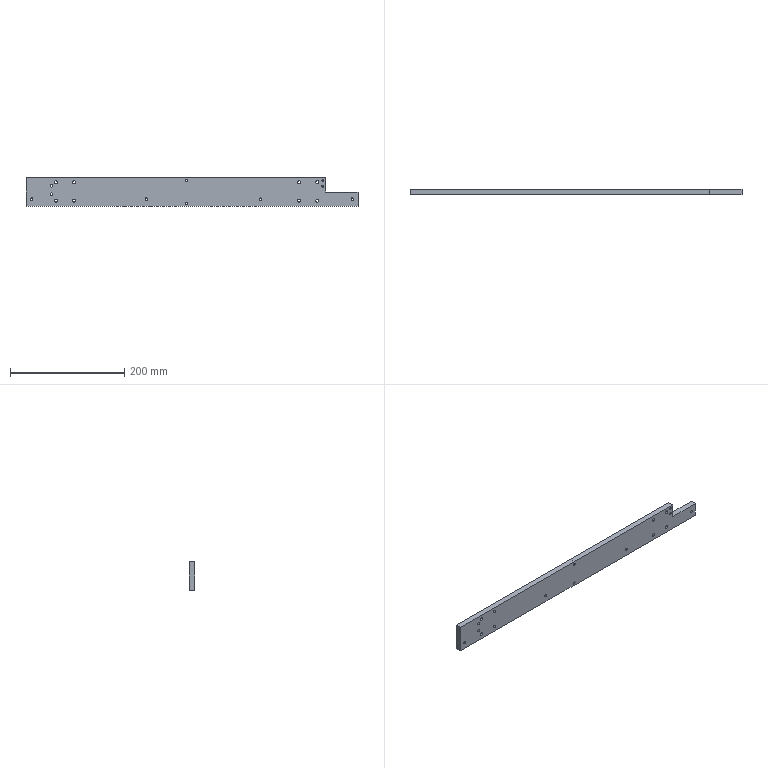Part | STEP file | 0243_219_Plate | 1 solid | 50 faces | box 580 x 10 x 50 mm | volume 272354 mm3 | cylinder 40 | plane 10 | commonest cylinder face diameters 5.5 x16 4.2 x8 3.3 x4 4.5 x4 5 x4 8 x4